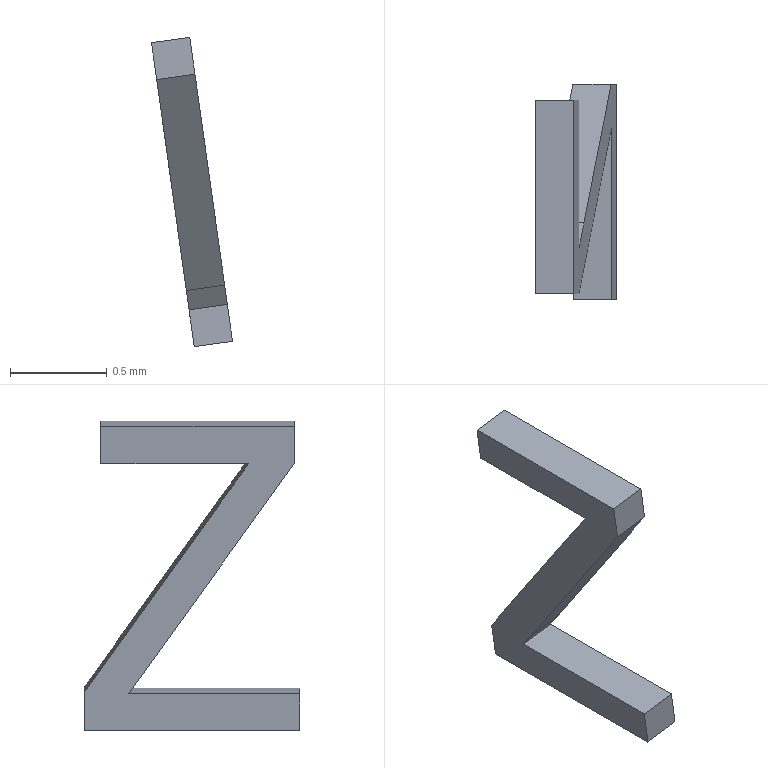Part | Creo | 1 solid | 14 faces | box 0.4191 x 1.116 x 1.601 mm | volume 0.1382 mm3 | plane 10 | other 3 | cylinder 1 | commonest cylinder face diameters 21.551 x1
STEP:
#1=CARTESIAN_POINT('',(-72.167,-123.05,-129.451));
#2=VERTEX_POINT('',#1);
#3=CARTESIAN_POINT('',(-72.026,-122.33,-130.453));
#4=VERTEX_POINT('',#3);
#5=CARTESIAN_POINT('',(-72.152,-122.97,-129.562));
#6=CARTESIAN_POINT('',(-72.12,-122.81,-129.785));
#7=CARTESIAN_POINT('',(-72.073,-122.57,-130.119));
#8=CARTESIAN_POINT('',(-72.042,-122.41,-130.341));
#9=B_SPLINE_CURVE_WITH_KNOTS('',3,(#1,#5,#6,#7,#8,#3),.UNSPECIFIED.,.F.,.F.,(4,1,1,4),(0.,0.3333,0.6667,1.),.UNSPECIFIED.);
#10=EDGE_CURVE('',#2,#4,#9,.T.);
#11=ORIENTED_EDGE('',*,*,#10,.T.);
#12=CARTESIAN_POINT('',(-71.828,-122.33,-130.425));
#13=VERTEX_POINT('',#12);
#14=CARTESIAN_POINT('',(-72.026,-122.33,-130.453));
#15=DIRECTION('',(0.9903,0.,0.1392));
#16=VECTOR('',#15,0.2);
#17=LINE('',#14,#16);
#18=EDGE_CURVE('',#4,#13,#17,.T.);
#19=ORIENTED_EDGE('',*,*,#18,.T.);
#20=CARTESIAN_POINT('',(-71.969,-123.05,-129.423));
#21=VERTEX_POINT('',#20);
#22=CARTESIAN_POINT('',(-71.844,-122.41,-130.313));
#23=CARTESIAN_POINT('',(-71.875,-122.57,-130.091));
#24=CARTESIAN_POINT('',(-71.922,-122.81,-129.757));
#25=CARTESIAN_POINT('',(-71.954,-122.97,-129.535));
#26=CARTESIAN_POINT('',(-71.969,-123.05,-129.423));
#27=B_SPLINE_CURVE_WITH_KNOTS('',3,(#12,#22,#23,#24,#25,#26),.UNSPECIFIED.,.F.,.F.,(4,1,1,4),(0.,0.3333,0.6667,1.),.UNSPECIFIED.);
#28=EDGE_CURVE('',#13,#21,#27,.T.);
#29=ORIENTED_EDGE('',*,*,#28,.T.);
#30=CARTESIAN_POINT('',(-72.167,-123.05,-129.451));
#31=DIRECTION('',(0.9903,0.,0.1392));
#32=VECTOR('',#31,0.2);
#33=LINE('',#30,#32);
#34=EDGE_CURVE('',#2,#21,#33,.T.);
#35=ORIENTED_EDGE('',*,*,#34,.F.);
#36=EDGE_LOOP('',(#11,#19,#29,#35));
#37=FACE_OUTER_BOUND('',#36,.F.);
#38=CARTESIAN_POINT('',(-71.827,-122.323,-130.435));
#39=CARTESIAN_POINT('',(-71.843,-122.405,-130.32));
#40=CARTESIAN_POINT('',(-71.875,-122.568,-130.094));
#41=CARTESIAN_POINT('',(-71.923,-122.812,-129.754));
#42=CARTESIAN_POINT('',(-71.954,-122.975,-129.528));
#43=CARTESIAN_POINT('',(-71.971,-123.057,-129.413));
#44=B_SPLINE_CURVE_WITH_KNOTS('',3,(#38,#39,#40,#41,#42,#43),.UNSPECIFIED.,.F.,.F.,(4,1,1,4),(0.,0.3366,0.6634,1.),.UNSPECIFIED.);
#45=DIRECTION('',(-0.9903,0.,-0.1392));
#46=VECTOR('',#45,1.);
#47=SURFACE_OF_LINEAR_EXTRUSION('',#44,#46);
#48=ADVANCED_FACE('',(#37),#47,.F.);
#49=ORIENTED_EDGE('',*,*,#10,.F.);
#50=CARTESIAN_POINT('',(-72.193,-123.181,-129.268));
#51=VERTEX_POINT('',#50);
#52=CARTESIAN_POINT('',(-73.049,-114.334,-123.176));
#53=DIRECTION('',(0.9903,0.,0.1392));
#54=DIRECTION('',(0.07945,-0.821,-0.5653));
#55=AXIS2_PLACEMENT_3D('',#52,#53,#54);
#56=CIRCLE('',#55,10.775);
#57=EDGE_CURVE('',#51,#2,#56,.T.);
#58=ORIENTED_EDGE('',*,*,#57,.F.);
#59=CARTESIAN_POINT('',(-72.193,-122.416,-129.268));
#60=VERTEX_POINT('',#59);
#61=CARTESIAN_POINT('',(-72.193,-122.416,-129.268));
#62=DIRECTION('',(0.,-1.,-0.000000002));
#63=VECTOR('',#62,0.7653);
#64=LINE('',#61,#63);
#65=EDGE_CURVE('',#60,#51,#64,.T.);
#66=ORIENTED_EDGE('',*,*,#65,.F.);
#67=CARTESIAN_POINT('',(-72.22,-122.416,-129.077));
#68=VERTEX_POINT('',#67);
#69=CARTESIAN_POINT('',(-72.193,-122.416,-129.268));
#70=DIRECTION('',(-0.1392,0.,0.9903));
#71=VECTOR('',#70,0.1929);
#72=LINE('',#69,#71);
#73=EDGE_CURVE('',#60,#68,#72,.T.);
#74=ORIENTED_EDGE('',*,*,#73,.T.);
#75=CARTESIAN_POINT('',(-72.22,-123.417,-129.077));
#76=VERTEX_POINT('',#75);
#77=CARTESIAN_POINT('',(-72.22,-123.417,-129.077));
#78=DIRECTION('',(0.,1.,0.));
#79=VECTOR('',#78,1.001);
#80=LINE('',#77,#79);
#81=EDGE_CURVE('',#76,#68,#80,.T.);
#82=ORIENTED_EDGE('',*,*,#81,.F.);
#83=CARTESIAN_POINT('',(-72.193,-123.417,-129.268));
#84=VERTEX_POINT('',#83);
#85=CARTESIAN_POINT('',(-72.22,-123.417,-129.077));
#86=DIRECTION('',(0.1392,0.,-0.9903));
#87=VECTOR('',#86,0.1929);
#88=LINE('',#85,#87);
#89=EDGE_CURVE('',#76,#84,#88,.T.);
#90=ORIENTED_EDGE('',*,*,#89,.T.);
#91=CARTESIAN_POINT('',(-72.04,-122.632,-130.359));
#92=VERTEX_POINT('',#91);
#93=CARTESIAN_POINT('',(-72.057,-122.719,-130.238));
#94=CARTESIAN_POINT('',(-72.091,-122.894,-129.995));
#95=CARTESIAN_POINT('',(-72.142,-123.155,-129.632));
#96=CARTESIAN_POINT('',(-72.176,-123.33,-129.389));
#97=CARTESIAN_POINT('',(-72.193,-123.417,-129.268));
#98=B_SPLINE_CURVE_WITH_KNOTS('',3,(#91,#93,#94,#95,#96,#97),.UNSPECIFIED.,.F.,.F.,(4,1,1,4),(0.,0.3334,0.6667,1.),.UNSPECIFIED.);
#99=EDGE_CURVE('',#92,#84,#98,.T.);
#100=ORIENTED_EDGE('',*,*,#99,.F.);
#101=CARTESIAN_POINT('',(-72.026,-122.56,-130.459));
#102=VERTEX_POINT('',#101);
#103=CARTESIAN_POINT('',(-72.027,-122.568,-130.448));
#104=CARTESIAN_POINT('',(-72.03,-122.584,-130.426));
#105=CARTESIAN_POINT('',(-72.035,-122.608,-130.392));
#106=CARTESIAN_POINT('',(-72.038,-122.624,-130.37));
#107=CARTESIAN_POINT('',(-72.04,-122.632,-130.359));
#108=B_SPLINE_CURVE_WITH_KNOTS('',3,(#101,#103,#104,#105,#106,#107),.UNSPECIFIED.,.F.,.F.,(4,1,1,4),(0.,0.3336,0.6664,1.),.UNSPECIFIED.);
#109=EDGE_CURVE('',#102,#92,#108,.T.);
#110=ORIENTED_EDGE('',*,*,#109,.F.);
#111=CARTESIAN_POINT('',(-72.026,-123.446,-130.459));
#112=VERTEX_POINT('',#111);
#113=CARTESIAN_POINT('',(-72.026,-123.446,-130.459));
#114=DIRECTION('',(0.,1.,0.));
#115=VECTOR('',#114,0.8859);
#116=LINE('',#113,#115);
#117=EDGE_CURVE('',#112,#102,#116,.T.);
#118=ORIENTED_EDGE('',*,*,#117,.F.);
#119=CARTESIAN_POINT('',(-71.999,-123.446,-130.65));
#120=VERTEX_POINT('',#119);
#121=CARTESIAN_POINT('',(-72.026,-123.446,-130.459));
#122=DIRECTION('',(0.1392,0.,-0.9903));
#123=VECTOR('',#122,0.1929);
#124=LINE('',#121,#123);
#125=EDGE_CURVE('',#112,#120,#124,.T.);
#126=ORIENTED_EDGE('',*,*,#125,.T.);
#127=CARTESIAN_POINT('',(-71.999,-122.33,-130.65));
#128=VERTEX_POINT('',#127);
#129=CARTESIAN_POINT('',(-71.999,-122.33,-130.65));
#130=DIRECTION('',(0.,-1.,0.));
#131=VECTOR('',#130,1.116);
#132=LINE('',#129,#131);
#133=EDGE_CURVE('',#128,#120,#132,.T.);
#134=ORIENTED_EDGE('',*,*,#133,.F.);
#135=CARTESIAN_POINT('',(-71.999,-122.33,-130.65));
#136=DIRECTION('',(-0.1392,0.,0.9903));
#137=VECTOR('',#136,0.1995);
#138=LINE('',#135,#137);
#139=EDGE_CURVE('',#128,#4,#138,.T.);
#140=ORIENTED_EDGE('',*,*,#139,.T.);
#141=EDGE_LOOP('',(#49,#58,#66,#74,#82,#90,#100,#110,#118,#126,#134,#140));
#142=FACE_OUTER_BOUND('',#141,.F.);
#143=CARTESIAN_POINT('',(-72.097,-122.69,-129.952));
#144=DIRECTION('',(-0.9903,0.,-0.1392));
#145=DIRECTION('',(-0.1392,0.,0.9903));
#146=AXIS2_PLACEMENT_3D('',#143,#144,#145);
#147=PLANE('',#146);
#148=ADVANCED_FACE('',(#142),#147,.T.);
#149=ORIENTED_EDGE('',*,*,#57,.T.);
#150=ORIENTED_EDGE('',*,*,#34,.T.);
#151=CARTESIAN_POINT('',(-71.995,-123.181,-129.24));
#152=VERTEX_POINT('',#151);
#153=CARTESIAN_POINT('',(-72.851,-114.334,-123.149));
#154=DIRECTION('',(-0.9903,0.,-0.1392));
#155=DIRECTION('',(0.08184,-0.8088,-0.5823));
#156=AXIS2_PLACEMENT_3D('',#153,#154,#155);
#157=CIRCLE('',#156,10.775);
#158=EDGE_CURVE('',#21,#152,#157,.T.);
#159=ORIENTED_EDGE('',*,*,#158,.T.);
#160=CARTESIAN_POINT('',(-72.193,-123.181,-129.268));
#161=DIRECTION('',(0.9903,0.,0.1392));
#162=VECTOR('',#161,0.2);
#163=LINE('',#160,#162);
#164=EDGE_CURVE('',#51,#152,#163,.T.);
#165=ORIENTED_EDGE('',*,*,#164,.F.);
#166=EDGE_LOOP('',(#149,#150,#159,#165));
#167=FACE_OUTER_BOUND('',#166,.F.);
#168=CARTESIAN_POINT('',(-72.851,-114.334,-123.149));
#169=DIRECTION('',(-0.9903,0.,-0.1392));
#170=DIRECTION('',(0.08184,-0.8088,-0.5823));
#171=AXIS2_PLACEMENT_3D('',#168,#169,#170);
#172=CYLINDRICAL_SURFACE('',#171,10.775);
#173=ADVANCED_FACE('',(#167),#172,.F.);
#174=ORIENTED_EDGE('',*,*,#28,.F.);
#175=CARTESIAN_POINT('',(-71.801,-122.33,-130.622));
#176=VERTEX_POINT('',#175);
#177=CARTESIAN_POINT('',(-71.828,-122.33,-130.425));
#178=DIRECTION('',(0.1392,0.,-0.9903));
#179=VECTOR('',#178,0.1995);
#180=LINE('',#177,#179);
#181=EDGE_CURVE('',#13,#176,#180,.T.);
#182=ORIENTED_EDGE('',*,*,#181,.T.);
#183=CARTESIAN_POINT('',(-71.801,-123.446,-130.622));
#184=VERTEX_POINT('',#183);
#185=CARTESIAN_POINT('',(-71.801,-122.33,-130.622));
#186=DIRECTION('',(0.,-1.,0.));
#187=VECTOR('',#186,1.116);
#188=LINE('',#185,#187);
#189=EDGE_CURVE('',#176,#184,#188,.T.);
#190=ORIENTED_EDGE('',*,*,#189,.T.);
#191=CARTESIAN_POINT('',(-71.827,-123.446,-130.431));
#192=VERTEX_POINT('',#191);
#193=CARTESIAN_POINT('',(-71.801,-123.446,-130.622));
#194=DIRECTION('',(-0.1392,0.,0.9903));
#195=VECTOR('',#194,0.1929);
#196=LINE('',#193,#195);
#197=EDGE_CURVE('',#184,#192,#196,.T.);
#198=ORIENTED_EDGE('',*,*,#197,.T.);
#199=CARTESIAN_POINT('',(-71.827,-122.56,-130.431));
#200=VERTEX_POINT('',#199);
#201=CARTESIAN_POINT('',(-71.827,-123.446,-130.431));
#202=DIRECTION('',(0.,1.,0.));
#203=VECTOR('',#202,0.8859);
#204=LINE('',#201,#203);
#205=EDGE_CURVE('',#192,#200,#204,.T.);
#206=ORIENTED_EDGE('',*,*,#205,.T.);
#207=CARTESIAN_POINT('',(-71.842,-122.632,-130.331));
#208=VERTEX_POINT('',#207);
#209=CARTESIAN_POINT('',(-71.842,-122.632,-130.331));
#210=CARTESIAN_POINT('',(-71.84,-122.624,-130.342));
#211=CARTESIAN_POINT('',(-71.837,-122.608,-130.365));
#212=CARTESIAN_POINT('',(-71.832,-122.584,-130.398));
#213=CARTESIAN_POINT('',(-71.829,-122.568,-130.42));
#214=CARTESIAN_POINT('',(-71.827,-122.56,-130.431));
#215=B_SPLINE_CURVE_WITH_KNOTS('',3,(#209,#210,#211,#212,#213,#214),.UNSPECIFIED.,.F.,.F.,(4,1,1,4),(0.,0.3336,0.6664,1.),.UNSPECIFIED.);
#216=EDGE_CURVE('',#208,#200,#215,.T.);
#217=ORIENTED_EDGE('',*,*,#216,.F.);
#218=CARTESIAN_POINT('',(-71.995,-123.417,-129.24));
#219=VERTEX_POINT('',#218);
#220=CARTESIAN_POINT('',(-71.995,-123.417,-129.24));
#221=CARTESIAN_POINT('',(-71.978,-123.33,-129.361));
#222=CARTESIAN_POINT('',(-71.944,-123.155,-129.604));
#223=CARTESIAN_POINT('',(-71.893,-122.894,-129.968));
#224=CARTESIAN_POINT('',(-71.859,-122.719,-130.21));
#225=CARTESIAN_POINT('',(-71.842,-122.632,-130.331));
#226=B_SPLINE_CURVE_WITH_KNOTS('',3,(#220,#221,#222,#223,#224,#225),.UNSPECIFIED.,.F.,.F.,(4,1,1,4),(0.,0.3333,0.6666,1.),.UNSPECIFIED.);
#227=EDGE_CURVE('',#219,#208,#226,.T.);
#228=ORIENTED_EDGE('',*,*,#227,.F.);
#229=CARTESIAN_POINT('',(-72.022,-123.417,-129.049));
#230=VERTEX_POINT('',#229);
#231=CARTESIAN_POINT('',(-71.995,-123.417,-129.24));
#232=DIRECTION('',(-0.1392,0.,0.9903));
#233=VECTOR('',#232,0.1929);
#234=LINE('',#231,#233);
#235=EDGE_CURVE('',#219,#230,#234,.T.);
#236=ORIENTED_EDGE('',*,*,#235,.T.);
#237=CARTESIAN_POINT('',(-72.022,-122.416,-129.049));
#238=VERTEX_POINT('',#237);
#239=CARTESIAN_POINT('',(-72.022,-123.417,-129.049));
#240=DIRECTION('',(0.,1.,0.));
#241=VECTOR('',#240,1.001);
#242=LINE('',#239,#241);
#243=EDGE_CURVE('',#230,#238,#242,.T.);
#244=ORIENTED_EDGE('',*,*,#243,.T.);
#245=CARTESIAN_POINT('',(-71.995,-122.416,-129.24));
#246=VERTEX_POINT('',#245);
#247=CARTESIAN_POINT('',(-72.022,-122.416,-129.049));
#248=DIRECTION('',(0.1392,0.,-0.9903));
#249=VECTOR('',#248,0.1929);
#250=LINE('',#247,#249);
#251=EDGE_CURVE('',#238,#246,#250,.T.);
#252=ORIENTED_EDGE('',*,*,#251,.T.);
#253=CARTESIAN_POINT('',(-71.995,-122.416,-129.24));
#254=DIRECTION('',(0.,-1.,-0.000000002));
#255=VECTOR('',#254,0.7653);
#256=LINE('',#253,#255);
#257=EDGE_CURVE('',#246,#152,#256,.T.);
#258=ORIENTED_EDGE('',*,*,#257,.T.);
#259=ORIENTED_EDGE('',*,*,#158,.F.);
#260=EDGE_LOOP('',(#174,#182,#190,#198,#206,#217,#228,#236,#244,#252,#258,#259));
#261=FACE_OUTER_BOUND('',#260,.F.);
#262=CARTESIAN_POINT('',(-71.899,-122.69,-129.924));
#263=DIRECTION('',(-0.9903,0.,-0.1392));
#264=DIRECTION('',(-0.1392,0.,0.9903));
#265=AXIS2_PLACEMENT_3D('',#262,#263,#264);
#266=PLANE('',#265);
#267=ADVANCED_FACE('',(#261),#266,.F.);
#268=ORIENTED_EDGE('',*,*,#139,.F.);
#269=CARTESIAN_POINT('',(-71.801,-122.33,-130.622));
#270=DIRECTION('',(-0.9903,0.,-0.1392));
#271=VECTOR('',#270,0.2);
#272=LINE('',#269,#271);
#273=EDGE_CURVE('',#176,#128,#272,.T.);
#274=ORIENTED_EDGE('',*,*,#273,.F.);
#275=ORIENTED_EDGE('',*,*,#181,.F.);
#276=ORIENTED_EDGE('',*,*,#18,.F.);
#277=EDGE_LOOP('',(#268,#274,#275,#276));
#278=FACE_OUTER_BOUND('',#277,.F.);
#279=CARTESIAN_POINT('',(-71.801,-122.33,-130.622));
#280=DIRECTION('',(0.,-1.,0.));
#281=DIRECTION('',(0.,0.,-1.));
#282=AXIS2_PLACEMENT_3D('',#279,#280,#281);
#283=PLANE('',#282);
#284=ADVANCED_FACE('',(#278),#283,.F.);
#285=ORIENTED_EDGE('',*,*,#133,.T.);
#286=CARTESIAN_POINT('',(-71.999,-123.446,-130.65));
#287=DIRECTION('',(0.9903,0.,0.1392));
#288=VECTOR('',#287,0.2);
#289=LINE('',#286,#288);
#290=EDGE_CURVE('',#120,#184,#289,.T.);
#291=ORIENTED_EDGE('',*,*,#290,.T.);
#292=ORIENTED_EDGE('',*,*,#189,.F.);
#293=ORIENTED_EDGE('',*,*,#273,.T.);
#294=EDGE_LOOP('',(#285,#291,#292,#293));
#295=FACE_OUTER_BOUND('',#294,.F.);
#296=CARTESIAN_POINT('',(-71.801,-123.446,-130.622));
#297=DIRECTION('',(-0.1392,0.,0.9903));
#298=DIRECTION('',(0.9903,0.,0.1392));
#299=AXIS2_PLACEMENT_3D('',#296,#297,#298);
#300=PLANE('',#299);
#301=ADVANCED_FACE('',(#295),#300,.F.);
#302=ORIENTED_EDGE('',*,*,#125,.F.);
#303=CARTESIAN_POINT('',(-71.827,-123.446,-130.431));
#304=DIRECTION('',(-0.9903,0.,-0.1392));
#305=VECTOR('',#304,0.2);
#306=LINE('',#303,#305);
#307=EDGE_CURVE('',#192,#112,#306,.T.);
#308=ORIENTED_EDGE('',*,*,#307,.F.);
#309=ORIENTED_EDGE('',*,*,#197,.F.);
#310=ORIENTED_EDGE('',*,*,#290,.F.);
#311=EDGE_LOOP('',(#302,#308,#309,#310));
#312=FACE_OUTER_BOUND('',#311,.F.);
#313=CARTESIAN_POINT('',(-71.827,-123.446,-130.431));
#314=DIRECTION('',(0.,1.,0.));
#315=DIRECTION('',(0.,0.,1.));
#316=AXIS2_PLACEMENT_3D('',#313,#314,#315);
#317=PLANE('',#316);
#318=ADVANCED_FACE('',(#312),#317,.F.);
#319=ORIENTED_EDGE('',*,*,#117,.T.);
#320=CARTESIAN_POINT('',(-72.026,-122.56,-130.459));
#321=DIRECTION('',(0.9903,0.,0.1392));
#322=VECTOR('',#321,0.2);
#323=LINE('',#320,#322);
#324=EDGE_CURVE('',#102,#200,#323,.T.);
#325=ORIENTED_EDGE('',*,*,#324,.T.);
#326=ORIENTED_EDGE('',*,*,#205,.F.);
#327=ORIENTED_EDGE('',*,*,#307,.T.);
#328=EDGE_LOOP('',(#319,#325,#326,#327));
#329=FACE_OUTER_BOUND('',#328,.F.);
#330=CARTESIAN_POINT('',(-71.827,-122.56,-130.431));
#331=DIRECTION('',(0.1392,0.,-0.9903));
#332=DIRECTION('',(-0.9903,0.,-0.1392));
#333=AXIS2_PLACEMENT_3D('',#330,#331,#332);
#334=PLANE('',#333);
#335=ADVANCED_FACE('',(#329),#334,.F.);
#336=ORIENTED_EDGE('',*,*,#109,.T.);
#337=CARTESIAN_POINT('',(-72.04,-122.632,-130.359));
#338=DIRECTION('',(0.9903,0.,0.1392));
#339=VECTOR('',#338,0.2);
#340=LINE('',#337,#339);
#341=EDGE_CURVE('',#92,#208,#340,.T.);
#342=ORIENTED_EDGE('',*,*,#341,.T.);
#343=ORIENTED_EDGE('',*,*,#216,.T.);
#344=ORIENTED_EDGE('',*,*,#324,.F.);
#345=EDGE_LOOP('',(#336,#342,#343,#344));
#346=FACE_OUTER_BOUND('',#345,.F.);
#347=CARTESIAN_POINT('',(-71.842,-122.633,-130.33));
#348=CARTESIAN_POINT('',(-71.84,-122.625,-130.342));
#349=CARTESIAN_POINT('',(-71.837,-122.608,-130.364));
#350=CARTESIAN_POINT('',(-71.832,-122.584,-130.398));
#351=CARTESIAN_POINT('',(-71.829,-122.567,-130.421));
#352=CARTESIAN_POINT('',(-71.827,-122.559,-130.432));
#353=B_SPLINE_CURVE_WITH_KNOTS('',3,(#347,#348,#349,#350,#351,#352),.UNSPECIFIED.,.F.,.F.,(4,1,1,4),(0.,0.3369,0.6631,1.),.UNSPECIFIED.);
#354=DIRECTION('',(-0.9903,0.,-0.1392));
#355=VECTOR('',#354,1.);
#356=SURFACE_OF_LINEAR_EXTRUSION('',#353,#355);
#357=ADVANCED_FACE('',(#346),#356,.F.);
#358=ORIENTED_EDGE('',*,*,#99,.T.);
#359=CARTESIAN_POINT('',(-72.193,-123.417,-129.268));
#360=DIRECTION('',(0.9903,0.,0.1392));
#361=VECTOR('',#360,0.2);
#362=LINE('',#359,#361);
#363=EDGE_CURVE('',#84,#219,#362,.T.);
#364=ORIENTED_EDGE('',*,*,#363,.T.);
#365=ORIENTED_EDGE('',*,*,#227,.T.);
#366=ORIENTED_EDGE('',*,*,#341,.F.);
#367=EDGE_LOOP('',(#358,#364,#365,#366));
#368=FACE_OUTER_BOUND('',#367,.F.);
#369=CARTESIAN_POINT('',(-71.996,-123.425,-129.229));
#370=CARTESIAN_POINT('',(-71.979,-123.335,-129.354));
#371=CARTESIAN_POINT('',(-71.944,-123.158,-129.6));
#372=CARTESIAN_POINT('',(-71.892,-122.891,-129.971));
#373=CARTESIAN_POINT('',(-71.858,-122.714,-130.217));
#374=CARTESIAN_POINT('',(-71.84,-122.624,-130.342));
#375=B_SPLINE_CURVE_WITH_KNOTS('',3,(#369,#370,#371,#372,#373,#374),.UNSPECIFIED.,.F.,.F.,(4,1,1,4),(0.,0.3366,0.6634,1.),.UNSPECIFIED.);
#376=DIRECTION('',(-0.9903,0.,-0.1392));
#377=VECTOR('',#376,1.);
#378=SURFACE_OF_LINEAR_EXTRUSION('',#375,#377);
#379=ADVANCED_FACE('',(#368),#378,.F.);
#380=ORIENTED_EDGE('',*,*,#89,.F.);
#381=CARTESIAN_POINT('',(-72.022,-123.417,-129.049));
#382=DIRECTION('',(-0.9903,0.,-0.1392));
#383=VECTOR('',#382,0.2);
#384=LINE('',#381,#383);
#385=EDGE_CURVE('',#230,#76,#384,.T.);
#386=ORIENTED_EDGE('',*,*,#385,.F.);
#387=ORIENTED_EDGE('',*,*,#235,.F.);
#388=ORIENTED_EDGE('',*,*,#363,.F.);
#389=EDGE_LOOP('',(#380,#386,#387,#388));
#390=FACE_OUTER_BOUND('',#389,.F.);
#391=CARTESIAN_POINT('',(-72.022,-123.417,-129.049));
#392=DIRECTION('',(0.,1.,0.));
#393=DIRECTION('',(0.,0.,1.));
#394=AXIS2_PLACEMENT_3D('',#391,#392,#393);
#395=PLANE('',#394);
#396=ADVANCED_FACE('',(#390),#395,.F.);
#397=ORIENTED_EDGE('',*,*,#81,.T.);
#398=CARTESIAN_POINT('',(-72.22,-122.416,-129.077));
#399=DIRECTION('',(0.9903,0.,0.1392));
#400=VECTOR('',#399,0.2);
#401=LINE('',#398,#400);
#402=EDGE_CURVE('',#68,#238,#401,.T.);
#403=ORIENTED_EDGE('',*,*,#402,.T.);
#404=ORIENTED_EDGE('',*,*,#243,.F.);
#405=ORIENTED_EDGE('',*,*,#385,.T.);
#406=EDGE_LOOP('',(#397,#403,#404,#405));
#407=FACE_OUTER_BOUND('',#406,.F.);
#408=CARTESIAN_POINT('',(-72.022,-122.416,-129.049));
#409=DIRECTION('',(0.1392,0.,-0.9903));
#410=DIRECTION('',(-0.9903,0.,-0.1392));
#411=AXIS2_PLACEMENT_3D('',#408,#409,#410);
#412=PLANE('',#411);
#413=ADVANCED_FACE('',(#407),#412,.F.);
#414=ORIENTED_EDGE('',*,*,#73,.F.);
#415=CARTESIAN_POINT('',(-71.995,-122.416,-129.24));
#416=DIRECTION('',(-0.9903,0.,-0.1392));
#417=VECTOR('',#416,0.2);
#418=LINE('',#415,#417);
#419=EDGE_CURVE('',#246,#60,#418,.T.);
#420=ORIENTED_EDGE('',*,*,#419,.F.);
#421=ORIENTED_EDGE('',*,*,#251,.F.);
#422=ORIENTED_EDGE('',*,*,#402,.F.);
#423=EDGE_LOOP('',(#414,#420,#421,#422));
#424=FACE_OUTER_BOUND('',#423,.F.);
#425=CARTESIAN_POINT('',(-71.995,-122.416,-129.24));
#426=DIRECTION('',(0.,-1.,0.));
#427=DIRECTION('',(0.,0.,-1.));
#428=AXIS2_PLACEMENT_3D('',#425,#426,#427);
#429=PLANE('',#428);
#430=ADVANCED_FACE('',(#424),#429,.F.);
#431=ORIENTED_EDGE('',*,*,#65,.T.);
#432=ORIENTED_EDGE('',*,*,#164,.T.);
#433=ORIENTED_EDGE('',*,*,#257,.F.);
#434=ORIENTED_EDGE('',*,*,#419,.T.);
#435=EDGE_LOOP('',(#431,#432,#433,#434));
#436=FACE_OUTER_BOUND('',#435,.F.);
#437=CARTESIAN_POINT('',(-71.995,-123.181,-129.24));
#438=DIRECTION('',(-0.1392,0.,0.9903));
#439=DIRECTION('',(0.9903,0.,0.1392));
#440=AXIS2_PLACEMENT_3D('',#437,#438,#439);
#441=PLANE('',#440);
#442=ADVANCED_FACE('',(#436),#441,.F.);
#443=CLOSED_SHELL('',(#48,#148,#173,#267,#284,#301,#318,#335,#357,#379,#396,#413,#430,#442));
#444=MANIFOLD_SOLID_BREP('',#443);
#445=(LENGTH_UNIT()NAMED_UNIT(*)SI_UNIT(.MILLI.,.METRE.));
#446=UNCERTAINTY_MEASURE_WITH_UNIT(LENGTH_MEASURE(0.0001996),#445,'','');
#447=(NAMED_UNIT(*)PLANE_ANGLE_UNIT()SI_UNIT($,.RADIAN.));
#448=PLANE_ANGLE_MEASURE_WITH_UNIT(PLANE_ANGLE_MEASURE(0.01745),#447);
#449=(CONVERSION_BASED_UNIT('DEGREE',#448)NAMED_UNIT(*)PLANE_ANGLE_UNIT());
#450=(NAMED_UNIT(*)SI_UNIT($,.STERADIAN.)SOLID_ANGLE_UNIT());
#451=(GEOMETRIC_REPRESENTATION_CONTEXT(3)GLOBAL_UNCERTAINTY_ASSIGNED_CONTEXT((#446))GLOBAL_UNIT_ASSIGNED_CONTEXT((#445,#449,#450))REPRESENTATION_CONTEXT('',''));
#452=ADVANCED_BREP_SHAPE_REPRESENTATION('',(#444),#451);